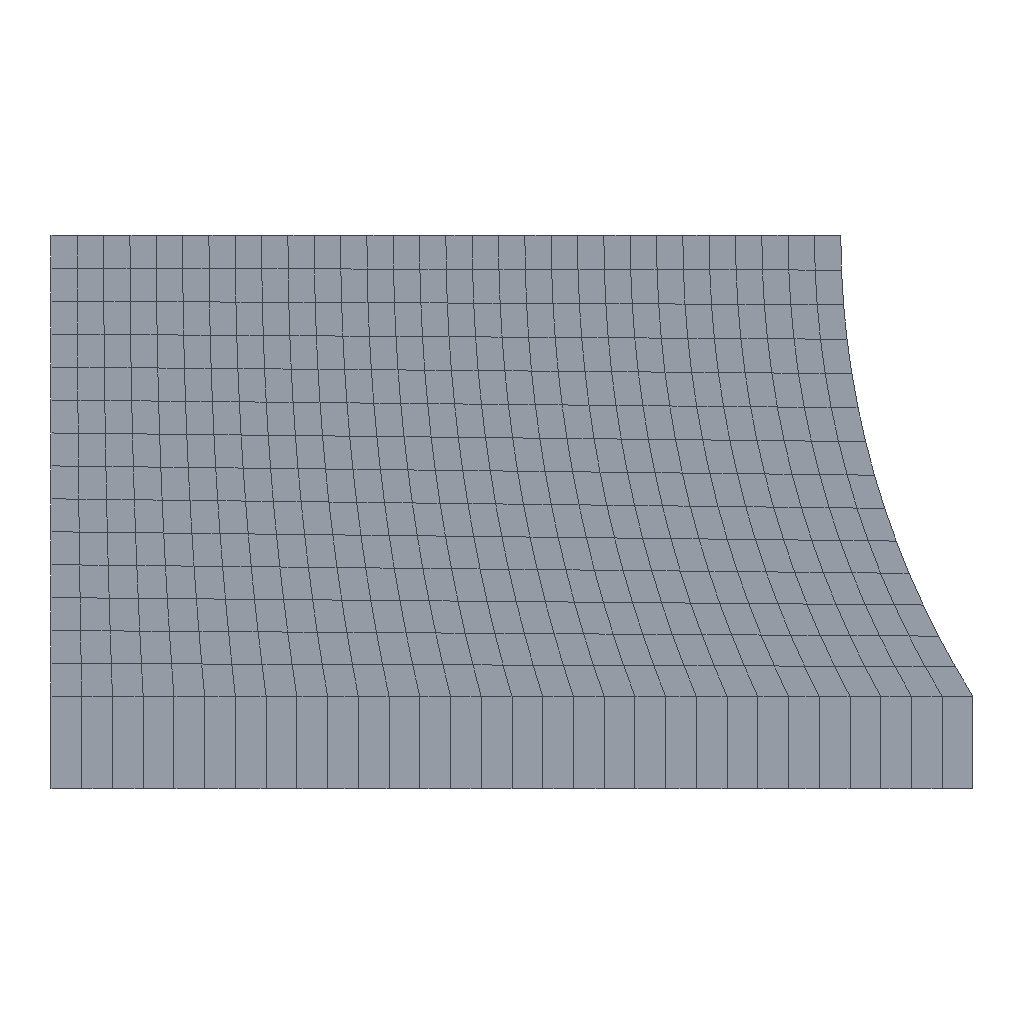Simulation study | abaqus
Set-up summary:
category,name,step,type,value,unit,region
solver,abaqus,,Abaqus/CAE 2024
units,SI m-kg-s (Pa),,inferred,E=2e+11 density=
analysis,Compress mount,,static,nlgeom=True; time_period=1
mesh,nodes,,,496
mesh,elements,,,450
element_type,CAX4H,,,420
element_type,CAX4I,,,30
material,Rubber,,behaviors,hyperelastic
material,Steel,,E,2e+11
material,Steel,,nu,0.3
section,Rubber,,solid section,,,_PickedSet3
section,Steel,,solid section,,,_PickedSet4
load,Pressure,Compress mount,pressure,500000,,Bottom
bc,Symmetry,Compress mount,fixed,[dofs=y],,Middle
Abaqus input file, long lists of numbers shortened:
*Heading
** Job name: deck Model name: Model-1
** Generated by: Abaqus/CAE 2024
*Preprint, echo=NO, model=NO, history=NO, contact=NO
**
** PARTS
**
*Part, name=Mount
*Node
      1, 0.01, 0.005
      2, 0.06, 0.005
** (494 more lines like these left out)
*Element, type=CAX4H
  1,   1,   7, 120,  90
  2,   7,   8, 121, 120
** (418 more lines like these left out)
*Element, type=CAX4I
421,   2,  35, 119,   6
422,  35,  34, 118, 119
** (28 more lines like these left out)
*Nset, nset=_PickedSet3, internal
   1,   2,   3,   4,   7,   8,   9,  10,  11,  12,  13,  14,  15,  16,  17,  18
  19,  20,  21,  22,  23,  24,  25,  26,  27,  28,  29,  30,  31,  32,  33,  34
** (28 more lines like these left out)
*Elset, elset=_PickedSet3, internal, generate
   1,  420,    1
*Nset, nset=_PickedSet4, internal
   1,   2,   5,   6,   7,   8,   9,  10,  11,  12,  13,  14,  15,  16,  17,  18
  19,  20,  21,  22,  23,  24,  25,  26,  27,  28,  29,  30,  31,  32,  33,  34
** (2 more lines like these left out)
*Elset, elset=_PickedSet4, internal, generate
 421,  450,    1
** Section: RubberSection
*Solid Section, elset=_PickedSet3, material=Rubber
1.,
** Section: SteelSection
*Solid Section, elset=_PickedSet4, material=Steel
1.,
*End Part
**
**
** ASSEMBLY
**
*Assembly, name=Assembly
**
*Instance, name=Mount-1, part=Mount
*End Instance
**
*Nset, nset=Middle, instance=Mount-1
  3,  4, 49, 50, 51, 52, 53, 54, 55, 56, 57, 58, 59, 60, 61, 62
 63, 64, 65, 66, 67, 68, 69, 70, 71, 72, 73, 74, 75, 76, 77
*Elset, elset=Middle, instance=Mount-1, generate
 391,  420,    1
*Nset, nset=Out, instance=Mount-1
 5,
*Elset, elset=_Bottom_S3, internal, instance=Mount-1, generate
 421,  450,    1
*Surface, type=ELEMENT, name=Bottom
_Bottom_S3, S3
*End Assembly
**
** MATERIALS
**
*Material, name=Rubber
*Hyperelastic, test data input
*Biaxial Test Data
    89000., 0.02
   255000., 0.14
   503000., 0.42
   958000., 1.49
 1.703e+06, 2.75
 2.413e+06, 3.45
*Planar Test Data
    55000.,  0.069
   324000., 0.2828
   758000., 1.386
 1.269e+06, 3.034
 1.779e+06, 4.062
*Uniaxial Test Data
 54000.,  0.038
152000., 0.1338
254000.,  0.221
362000.,  0.345
459000.,   0.46
583000., 0.6242
656000.,  0.851
730000., 1.427
*Material, name=Steel
*Elastic
 2e+11, 0.3
** ----------------------------------------------------------------
**
** STEP: Compress mount
**
*Step, name="Compress mount", nlgeom=YES
Apply axial pressure load to mount
*Static
0.01, 1., 1e-05, 1.
**
** BOUNDARY CONDITIONS
**
** Name: Symmetry Type: Displacement/Rotation
*Boundary
Middle, 2, 2
**
** LOADS
**
** Name: Pressure   Type: Pressure
*Dsload
Bottom, P, 500000.
**
** OUTPUT REQUESTS
**
*Restart, write, frequency=0
**
** FIELD OUTPUT: F-Output-1
**
*Output, field
*Node Output
CF, RF, U
*Element Output, directions=YES
LE, NE, PE, PEEQ, PEMAG, S
*Contact Output
CDISP, CSTRESS
**
** HISTORY OUTPUT: H-Output-1
**
*Output, history
*Node Output, nset=Out
U1, U2, U3
*End Step
Results summary:
result,odb.job_status,,,JOB_STATUS_COMPLETED_SUCCESSFULLY,"consistent, unstated (Abaqus has no unit system)"
result,steps[0].procedure,Compress mount,,*STATIC,"consistent, unstated (Abaqus has no unit system)"
result,steps[0].time_period,Compress mount,,1,"consistent, unstated (Abaqus has no unit system)"
result,steps[0].n_frames,Compress mount,,12,"consistent, unstated (Abaqus has no unit system)"
result,steps[0].last_frame.id,Compress mount,,11,"consistent, unstated (Abaqus has no unit system)"
result,steps[0].last_frame.value,Compress mount,,1,"consistent, unstated (Abaqus has no unit system)"
result,steps[0].last_frame.description,Compress mount,,Increment     11: Step Time =    1.000,"consistent, unstated (Abaqus has no unit system)"
result,steps[0].completed,Compress mount,,True,"consistent, unstated (Abaqus has no unit system)"
result,steps[0].max_U_magnitude,Compress mount,,0.009476,"consistent, unstated (Abaqus has no unit system)"
result,steps[0].max_S_mises,Compress mount,,8.56817e+06,"consistent, unstated (Abaqus has no unit system)"
result,steps[0].RF_sum[1],Compress mount,,0,"consistent, unstated (Abaqus has no unit system)"
result,steps[0].RF_sum[2],Compress mount,,-5497.61,"consistent, unstated (Abaqus has no unit system)"